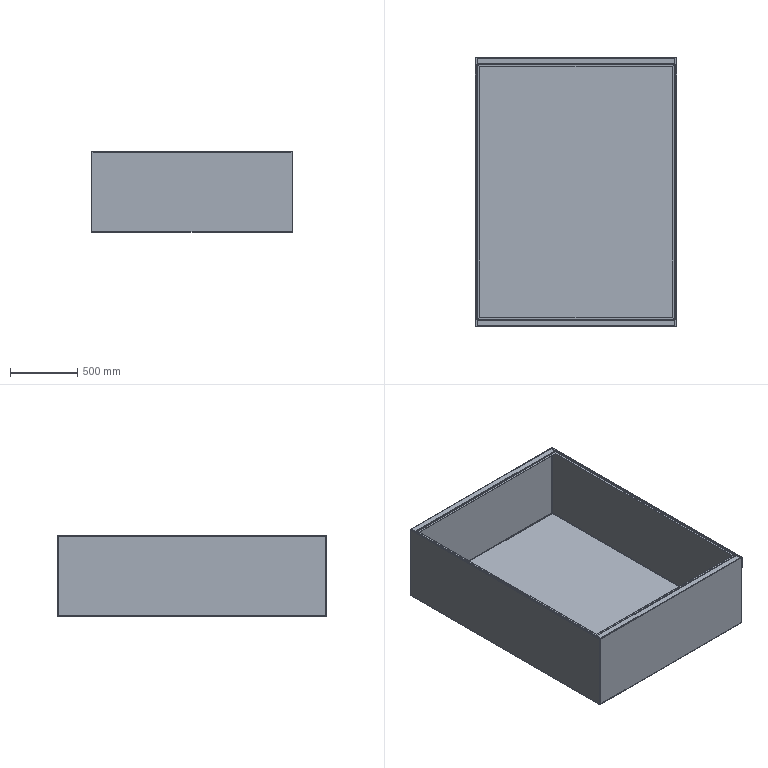Part | SolidWorks | features EdgeFlange 6, FlatPattern 1, SMBaseFlange 1, SheetMetal 1, WeldmentFeature 1 | 1 solid | 166 faces | box 1500 x 2000 x 600 mm | volume 14989155 mm3 | plane 118 | cylinder 32 | spline 16 | commonest cylinder face diameters 4 x12 8 x12 1.473 x4 5.473 x4